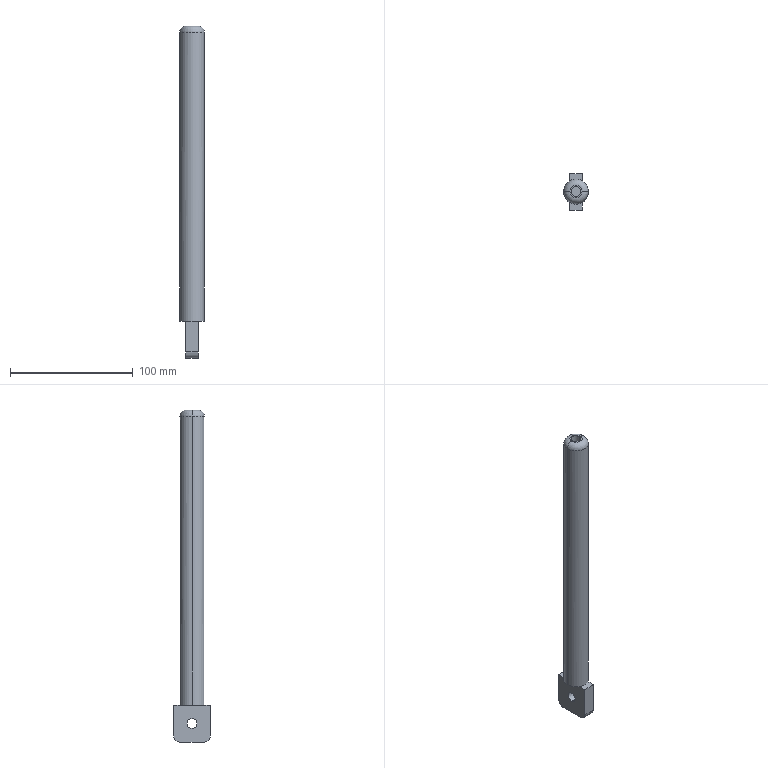Part | SolidWorks | features ICE 3, Fillet 2, Extrusion 1 | 1 solid | 21 faces | box 20 x 30 x 270 mm | volume 82484 mm3 | plane 11 | cylinder 8 | torus 2 | commonest cylinder face diameters 8 x4 10 x2 20 x2
STEP:
#1=CARTESIAN_POINT('',(-4.,0.,220.));
#2=VERTEX_POINT('',#1);
#3=CARTESIAN_POINT('',(4.,0.,220.));
#4=VERTEX_POINT('',#3);
#5=CARTESIAN_POINT('',(0.,0.,220.));
#6=DIRECTION('',(0.,0.,1.));
#7=DIRECTION('',(1.,0.,0.));
#8=AXIS2_PLACEMENT_3D('',#5,#6,#7);
#9=CIRCLE('',#8,4.);
#10=EDGE_CURVE('',#2,#4,#9,.T.);
#11=ORIENTED_EDGE('',*,*,#10,.F.);
#12=CARTESIAN_POINT('',(-4.,0.,240.));
#13=VERTEX_POINT('',#12);
#14=CARTESIAN_POINT('',(-4.,0.,220.));
#15=DIRECTION('',(0.,0.,1.));
#16=VECTOR('',#15,1000.);
#17=LINE('',#14,#16);
#18=EDGE_CURVE('',#2,#13,#17,.T.);
#19=ORIENTED_EDGE('',*,*,#18,.T.);
#20=CARTESIAN_POINT('',(4.,0.,240.));
#21=VERTEX_POINT('',#20);
#22=CARTESIAN_POINT('',(0.,0.,240.));
#23=DIRECTION('',(0.,0.,1.));
#24=DIRECTION('',(1.,0.,0.));
#25=AXIS2_PLACEMENT_3D('',#22,#23,#24);
#26=CIRCLE('',#25,4.);
#27=EDGE_CURVE('',#13,#21,#26,.T.);
#28=ORIENTED_EDGE('',*,*,#27,.T.);
#29=CARTESIAN_POINT('',(4.,0.,220.));
#30=DIRECTION('',(0.,0.,1.));
#31=VECTOR('',#30,1000.);
#32=LINE('',#29,#31);
#33=EDGE_CURVE('',#4,#21,#32,.T.);
#34=ORIENTED_EDGE('',*,*,#33,.F.);
#35=EDGE_LOOP('',(#11,#19,#28,#34));
#36=FACE_OUTER_BOUND('',#35,.T.);
#37=CARTESIAN_POINT('',(0.,0.,220.));
#38=DIRECTION('',(0.,0.,1.));
#39=DIRECTION('',(1.,0.,0.));
#40=AXIS2_PLACEMENT_3D('',#37,#38,#39);
#41=CYLINDRICAL_SURFACE('',#40,4.);
#42=ADVANCED_FACE('',(#36),#41,.F.);
#43=CARTESIAN_POINT('',(-10.,0.,235.));
#44=VERTEX_POINT('',#43);
#45=CARTESIAN_POINT('',(10.,0.,235.));
#46=VERTEX_POINT('',#45);
#47=CARTESIAN_POINT('',(0.,0.,235.));
#48=DIRECTION('',(0.,0.,-1.));
#49=DIRECTION('',(1.,0.,0.));
#50=AXIS2_PLACEMENT_3D('',#47,#48,#49);
#51=CIRCLE('',#50,10.);
#52=EDGE_CURVE('',#44,#46,#51,.T.);
#53=ORIENTED_EDGE('',*,*,#52,.F.);
#54=CARTESIAN_POINT('',(-5.,0.,240.));
#55=VERTEX_POINT('',#54);
#56=CARTESIAN_POINT('',(-5.,0.,235.));
#57=DIRECTION('',(0.,1.,0.));
#58=DIRECTION('',(-1.,0.,0.));
#59=AXIS2_PLACEMENT_3D('',#56,#57,#58);
#60=CIRCLE('',#59,5.);
#61=EDGE_CURVE('',#44,#55,#60,.T.);
#62=ORIENTED_EDGE('',*,*,#61,.T.);
#63=CARTESIAN_POINT('',(5.,0.,240.));
#64=VERTEX_POINT('',#63);
#65=CARTESIAN_POINT('',(0.,0.,240.));
#66=DIRECTION('',(0.,0.,1.));
#67=DIRECTION('',(1.,0.,0.));
#68=AXIS2_PLACEMENT_3D('',#65,#66,#67);
#69=CIRCLE('',#68,5.);
#70=EDGE_CURVE('',#64,#55,#69,.T.);
#71=ORIENTED_EDGE('',*,*,#70,.F.);
#72=CARTESIAN_POINT('',(5.,0.,235.));
#73=DIRECTION('',(0.,-1.,0.));
#74=DIRECTION('',(0.,0.,-1.));
#75=AXIS2_PLACEMENT_3D('',#72,#73,#74);
#76=CIRCLE('',#75,5.);
#77=EDGE_CURVE('',#46,#64,#76,.T.);
#78=ORIENTED_EDGE('',*,*,#77,.F.);
#79=EDGE_LOOP('',(#53,#62,#71,#78));
#80=FACE_OUTER_BOUND('',#79,.T.);
#81=CARTESIAN_POINT('',(0.,0.,235.));
#82=DIRECTION('',(0.,0.,1.));
#83=DIRECTION('',(1.,0.,0.));
#84=AXIS2_PLACEMENT_3D('',#81,#82,#83);
#85=TOROIDAL_SURFACE('',#84,5.,5.);
#86=ADVANCED_FACE('',(#80),#85,.T.);
#87=CARTESIAN_POINT('',(-5.,0.,-19.));
#88=VERTEX_POINT('',#87);
#89=CARTESIAN_POINT('',(-5.,0.,-11.));
#90=VERTEX_POINT('',#89);
#91=CARTESIAN_POINT('',(-5.,0.,-15.));
#92=DIRECTION('',(-1.,0.,0.));
#93=DIRECTION('',(0.,0.,1.));
#94=AXIS2_PLACEMENT_3D('',#91,#92,#93);
#95=CIRCLE('',#94,4.);
#96=EDGE_CURVE('',#88,#90,#95,.T.);
#97=ORIENTED_EDGE('',*,*,#96,.T.);
#98=CARTESIAN_POINT('',(5.,0.,-11.));
#99=VERTEX_POINT('',#98);
#100=CARTESIAN_POINT('',(-33.,0.,-11.));
#101=DIRECTION('',(1.,0.,0.));
#102=VECTOR('',#101,1000.);
#103=LINE('',#100,#102);
#104=EDGE_CURVE('',#90,#99,#103,.T.);
#105=ORIENTED_EDGE('',*,*,#104,.T.);
#106=CARTESIAN_POINT('',(5.,0.,-19.));
#107=VERTEX_POINT('',#106);
#108=CARTESIAN_POINT('',(5.,0.,-15.));
#109=DIRECTION('',(1.,0.,0.));
#110=DIRECTION('',(0.,0.,-1.));
#111=AXIS2_PLACEMENT_3D('',#108,#109,#110);
#112=CIRCLE('',#111,4.);
#113=EDGE_CURVE('',#99,#107,#112,.T.);
#114=ORIENTED_EDGE('',*,*,#113,.T.);
#115=CARTESIAN_POINT('',(-33.,0.,-19.));
#116=DIRECTION('',(1.,0.,0.));
#117=VECTOR('',#116,1000.);
#118=LINE('',#115,#117);
#119=EDGE_CURVE('',#88,#107,#118,.T.);
#120=ORIENTED_EDGE('',*,*,#119,.F.);
#121=EDGE_LOOP('',(#97,#105,#114,#120));
#122=FACE_OUTER_BOUND('',#121,.T.);
#123=CARTESIAN_POINT('',(-33.,0.,-15.));
#124=DIRECTION('',(1.,0.,0.));
#125=DIRECTION('',(0.,0.,-1.));
#126=AXIS2_PLACEMENT_3D('',#123,#124,#125);
#127=CYLINDRICAL_SURFACE('',#126,4.);
#128=ADVANCED_FACE('',(#122),#127,.F.);
#129=ORIENTED_EDGE('',*,*,#52,.T.);
#130=CARTESIAN_POINT('',(10.,0.,0.));
#131=VERTEX_POINT('',#130);
#132=CARTESIAN_POINT('',(10.,0.,240.));
#133=DIRECTION('',(0.,0.,-1.));
#134=VECTOR('',#133,1000.);
#135=LINE('',#132,#134);
#136=EDGE_CURVE('',#46,#131,#135,.T.);
#137=ORIENTED_EDGE('',*,*,#136,.T.);
#138=CARTESIAN_POINT('',(5.,8.66,0.));
#139=VERTEX_POINT('',#138);
#140=CARTESIAN_POINT('',(0.,0.,0.));
#141=DIRECTION('',(0.,0.,1.));
#142=DIRECTION('',(1.,0.,0.));
#143=AXIS2_PLACEMENT_3D('',#140,#141,#142);
#144=CIRCLE('',#143,10.);
#145=EDGE_CURVE('',#131,#139,#144,.T.);
#146=ORIENTED_EDGE('',*,*,#145,.T.);
#147=CARTESIAN_POINT('',(-5.,8.66,0.));
#148=VERTEX_POINT('',#147);
#149=CARTESIAN_POINT('',(0.,0.,0.));
#150=DIRECTION('',(0.,0.,1.));
#151=DIRECTION('',(1.,0.,0.));
#152=AXIS2_PLACEMENT_3D('',#149,#150,#151);
#153=CIRCLE('',#152,10.);
#154=EDGE_CURVE('',#139,#148,#153,.T.);
#155=ORIENTED_EDGE('',*,*,#154,.T.);
#156=CARTESIAN_POINT('',(-10.,0.,0.));
#157=VERTEX_POINT('',#156);
#158=CARTESIAN_POINT('',(0.,0.,0.));
#159=DIRECTION('',(0.,0.,1.));
#160=DIRECTION('',(1.,0.,0.));
#161=AXIS2_PLACEMENT_3D('',#158,#159,#160);
#162=CIRCLE('',#161,10.);
#163=EDGE_CURVE('',#148,#157,#162,.T.);
#164=ORIENTED_EDGE('',*,*,#163,.T.);
#165=CARTESIAN_POINT('',(-10.,0.,240.));
#166=DIRECTION('',(0.,0.,-1.));
#167=VECTOR('',#166,1000.);
#168=LINE('',#165,#167);
#169=EDGE_CURVE('',#44,#157,#168,.T.);
#170=ORIENTED_EDGE('',*,*,#169,.F.);
#171=EDGE_LOOP('',(#129,#137,#146,#155,#164,#170));
#172=FACE_OUTER_BOUND('',#171,.T.);
#173=CARTESIAN_POINT('',(0.,0.,240.));
#174=DIRECTION('',(0.,0.,-1.));
#175=DIRECTION('',(-1.,0.,0.));
#176=AXIS2_PLACEMENT_3D('',#173,#174,#175);
#177=CYLINDRICAL_SURFACE('',#176,10.);
#178=ADVANCED_FACE('',(#172),#177,.T.);
#179=CARTESIAN_POINT('',(5.,-8.66,0.));
#180=VERTEX_POINT('',#179);
#181=CARTESIAN_POINT('',(5.,-15.,0.));
#182=DIRECTION('',(0.,-1.,0.));
#183=VECTOR('',#182,1000.);
#184=LINE('',#181,#183);
#185=EDGE_CURVE('',#139,#180,#184,.T.);
#186=ORIENTED_EDGE('',*,*,#185,.F.);
#187=ORIENTED_EDGE('',*,*,#145,.F.);
#188=CARTESIAN_POINT('',(0.,0.,0.));
#189=DIRECTION('',(0.,0.,1.));
#190=DIRECTION('',(1.,0.,0.));
#191=AXIS2_PLACEMENT_3D('',#188,#189,#190);
#192=CIRCLE('',#191,10.);
#193=EDGE_CURVE('',#180,#131,#192,.T.);
#194=ORIENTED_EDGE('',*,*,#193,.F.);
#195=EDGE_LOOP('',(#186,#187,#194));
#196=FACE_OUTER_BOUND('',#195,.T.);
#197=CARTESIAN_POINT('',(0.,0.,0.));
#198=DIRECTION('',(0.,0.,1.));
#199=DIRECTION('',(1.,0.,0.));
#200=AXIS2_PLACEMENT_3D('',#197,#198,#199);
#201=PLANE('',#200);
#202=ADVANCED_FACE('',(#196),#201,.F.);
#203=ORIENTED_EDGE('',*,*,#136,.F.);
#204=CARTESIAN_POINT('',(0.,0.,235.));
#205=DIRECTION('',(0.,0.,-1.));
#206=DIRECTION('',(1.,0.,0.));
#207=AXIS2_PLACEMENT_3D('',#204,#205,#206);
#208=CIRCLE('',#207,10.);
#209=EDGE_CURVE('',#46,#44,#208,.T.);
#210=ORIENTED_EDGE('',*,*,#209,.T.);
#211=ORIENTED_EDGE('',*,*,#169,.T.);
#212=CARTESIAN_POINT('',(-5.,-8.66,0.));
#213=VERTEX_POINT('',#212);
#214=CARTESIAN_POINT('',(0.,0.,0.));
#215=DIRECTION('',(0.,0.,1.));
#216=DIRECTION('',(1.,0.,0.));
#217=AXIS2_PLACEMENT_3D('',#214,#215,#216);
#218=CIRCLE('',#217,10.);
#219=EDGE_CURVE('',#157,#213,#218,.T.);
#220=ORIENTED_EDGE('',*,*,#219,.T.);
#221=CARTESIAN_POINT('',(0.,0.,0.));
#222=DIRECTION('',(0.,0.,1.));
#223=DIRECTION('',(1.,0.,0.));
#224=AXIS2_PLACEMENT_3D('',#221,#222,#223);
#225=CIRCLE('',#224,10.);
#226=EDGE_CURVE('',#213,#180,#225,.T.);
#227=ORIENTED_EDGE('',*,*,#226,.T.);
#228=ORIENTED_EDGE('',*,*,#193,.T.);
#229=EDGE_LOOP('',(#203,#210,#211,#220,#227,#228));
#230=FACE_OUTER_BOUND('',#229,.T.);
#231=CARTESIAN_POINT('',(0.,0.,240.));
#232=DIRECTION('',(0.,0.,-1.));
#233=DIRECTION('',(-1.,0.,0.));
#234=AXIS2_PLACEMENT_3D('',#231,#232,#233);
#235=CYLINDRICAL_SURFACE('',#234,10.);
#236=ADVANCED_FACE('',(#230),#235,.T.);
#237=CARTESIAN_POINT('',(0.,0.,240.));
#238=DIRECTION('',(0.,0.,1.));
#239=DIRECTION('',(1.,0.,0.));
#240=AXIS2_PLACEMENT_3D('',#237,#238,#239);
#241=CIRCLE('',#240,4.);
#242=EDGE_CURVE('',#21,#13,#241,.T.);
#243=ORIENTED_EDGE('',*,*,#242,.F.);
#244=ORIENTED_EDGE('',*,*,#27,.F.);
#245=EDGE_LOOP('',(#243,#244));
#246=FACE_BOUND('',#245,.T.);
#247=ORIENTED_EDGE('',*,*,#70,.T.);
#248=CARTESIAN_POINT('',(0.,0.,240.));
#249=DIRECTION('',(0.,0.,1.));
#250=DIRECTION('',(1.,0.,0.));
#251=AXIS2_PLACEMENT_3D('',#248,#249,#250);
#252=CIRCLE('',#251,5.);
#253=EDGE_CURVE('',#55,#64,#252,.T.);
#254=ORIENTED_EDGE('',*,*,#253,.T.);
#255=EDGE_LOOP('',(#247,#254));
#256=FACE_OUTER_BOUND('',#255,.T.);
#257=CARTESIAN_POINT('',(0.,0.,240.));
#258=DIRECTION('',(0.,0.,1.));
#259=DIRECTION('',(1.,0.,0.));
#260=AXIS2_PLACEMENT_3D('',#257,#258,#259);
#261=PLANE('',#260);
#262=ADVANCED_FACE('',(#246,#256),#261,.T.);
#263=ORIENTED_EDGE('',*,*,#163,.F.);
#264=CARTESIAN_POINT('',(-5.,-15.,0.));
#265=DIRECTION('',(0.,-1.,0.));
#266=VECTOR('',#265,1000.);
#267=LINE('',#264,#266);
#268=EDGE_CURVE('',#148,#213,#267,.T.);
#269=ORIENTED_EDGE('',*,*,#268,.T.);
#270=ORIENTED_EDGE('',*,*,#219,.F.);
#271=EDGE_LOOP('',(#263,#269,#270));
#272=FACE_OUTER_BOUND('',#271,.T.);
#273=CARTESIAN_POINT('',(0.,0.,0.));
#274=DIRECTION('',(0.,0.,1.));
#275=DIRECTION('',(1.,0.,0.));
#276=AXIS2_PLACEMENT_3D('',#273,#274,#275);
#277=PLANE('',#276);
#278=ADVANCED_FACE('',(#272),#277,.F.);
#279=ORIENTED_EDGE('',*,*,#154,.F.);
#280=CARTESIAN_POINT('',(5.,15.,0.));
#281=VERTEX_POINT('',#280);
#282=CARTESIAN_POINT('',(5.,-15.,0.));
#283=DIRECTION('',(0.,-1.,0.));
#284=VECTOR('',#283,1000.);
#285=LINE('',#282,#284);
#286=EDGE_CURVE('',#281,#139,#285,.T.);
#287=ORIENTED_EDGE('',*,*,#286,.F.);
#288=CARTESIAN_POINT('',(-5.,15.,0.));
#289=VERTEX_POINT('',#288);
#290=CARTESIAN_POINT('',(5.,15.,0.));
#291=DIRECTION('',(-1.,0.,0.));
#292=VECTOR('',#291,1000.);
#293=LINE('',#290,#292);
#294=EDGE_CURVE('',#281,#289,#293,.T.);
#295=ORIENTED_EDGE('',*,*,#294,.T.);
#296=CARTESIAN_POINT('',(-5.,-15.,0.));
#297=DIRECTION('',(0.,-1.,0.));
#298=VECTOR('',#297,1000.);
#299=LINE('',#296,#298);
#300=EDGE_CURVE('',#289,#148,#299,.T.);
#301=ORIENTED_EDGE('',*,*,#300,.T.);
#302=EDGE_LOOP('',(#279,#287,#295,#301));
#303=FACE_OUTER_BOUND('',#302,.T.);
#304=CARTESIAN_POINT('',(5.,-15.,0.));
#305=DIRECTION('',(0.,0.,-1.));
#306=DIRECTION('',(-1.,0.,0.));
#307=AXIS2_PLACEMENT_3D('',#304,#305,#306);
#308=PLANE('',#307);
#309=ADVANCED_FACE('',(#303),#308,.F.);
#310=CARTESIAN_POINT('',(-5.,-10.,-30.));
#311=VERTEX_POINT('',#310);
#312=CARTESIAN_POINT('',(-5.,10.,-30.));
#313=VERTEX_POINT('',#312);
#314=CARTESIAN_POINT('',(-5.,-15.,-30.));
#315=DIRECTION('',(0.,1.,0.));
#316=VECTOR('',#315,1000.);
#317=LINE('',#314,#316);
#318=EDGE_CURVE('',#311,#313,#317,.T.);
#319=ORIENTED_EDGE('',*,*,#318,.T.);
#320=CARTESIAN_POINT('',(5.,10.,-30.));
#321=VERTEX_POINT('',#320);
#322=CARTESIAN_POINT('',(5.,10.,-30.));
#323=DIRECTION('',(1.,0.,0.));
#324=VECTOR('',#323,1000.);
#325=LINE('',#322,#324);
#326=EDGE_CURVE('',#313,#321,#325,.T.);
#327=ORIENTED_EDGE('',*,*,#326,.T.);
#328=CARTESIAN_POINT('',(5.,-10.,-30.));
#329=VERTEX_POINT('',#328);
#330=CARTESIAN_POINT('',(5.,-15.,-30.));
#331=DIRECTION('',(0.,1.,0.));
#332=VECTOR('',#331,1000.);
#333=LINE('',#330,#332);
#334=EDGE_CURVE('',#329,#321,#333,.T.);
#335=ORIENTED_EDGE('',*,*,#334,.F.);
#336=CARTESIAN_POINT('',(5.,-10.,-30.));
#337=DIRECTION('',(-1.,0.,0.));
#338=VECTOR('',#337,1000.);
#339=LINE('',#336,#338);
#340=EDGE_CURVE('',#329,#311,#339,.T.);
#341=ORIENTED_EDGE('',*,*,#340,.T.);
#342=EDGE_LOOP('',(#319,#327,#335,#341));
#343=FACE_OUTER_BOUND('',#342,.T.);
#344=CARTESIAN_POINT('',(5.,-15.,-30.));
#345=DIRECTION('',(0.,0.,1.));
#346=DIRECTION('',(1.,0.,0.));
#347=AXIS2_PLACEMENT_3D('',#344,#345,#346);
#348=PLANE('',#347);
#349=ADVANCED_FACE('',(#343),#348,.F.);
#350=CARTESIAN_POINT('',(5.,15.,-25.));
#351=VERTEX_POINT('',#350);
#352=CARTESIAN_POINT('',(5.,15.,0.));
#353=DIRECTION('',(0.,0.,1.));
#354=VECTOR('',#353,1000.);
#355=LINE('',#352,#354);
#356=EDGE_CURVE('',#351,#281,#355,.T.);
#357=ORIENTED_EDGE('',*,*,#356,.F.);
#358=CARTESIAN_POINT('',(-5.,15.,-25.));
#359=VERTEX_POINT('',#358);
#360=CARTESIAN_POINT('',(5.,15.,-25.));
#361=DIRECTION('',(-1.,0.,0.));
#362=VECTOR('',#361,1000.);
#363=LINE('',#360,#362);
#364=EDGE_CURVE('',#351,#359,#363,.T.);
#365=ORIENTED_EDGE('',*,*,#364,.T.);
#366=CARTESIAN_POINT('',(-5.,15.,0.));
#367=DIRECTION('',(0.,0.,1.));
#368=VECTOR('',#367,1000.);
#369=LINE('',#366,#368);
#370=EDGE_CURVE('',#359,#289,#369,.T.);
#371=ORIENTED_EDGE('',*,*,#370,.T.);
#372=ORIENTED_EDGE('',*,*,#294,.F.);
#373=EDGE_LOOP('',(#357,#365,#371,#372));
#374=FACE_OUTER_BOUND('',#373,.T.);
#375=CARTESIAN_POINT('',(5.,15.,0.));
#376=DIRECTION('',(0.,-1.,0.));
#377=DIRECTION('',(0.,0.,-1.));
#378=AXIS2_PLACEMENT_3D('',#375,#376,#377);
#379=PLANE('',#378);
#380=ADVANCED_FACE('',(#374),#379,.F.);
#381=ORIENTED_EDGE('',*,*,#226,.F.);
#382=CARTESIAN_POINT('',(-5.,-15.,0.));
#383=VERTEX_POINT('',#382);
#384=CARTESIAN_POINT('',(-5.,-15.,0.));
#385=DIRECTION('',(0.,-1.,0.));
#386=VECTOR('',#385,1000.);
#387=LINE('',#384,#386);
#388=EDGE_CURVE('',#213,#383,#387,.T.);
#389=ORIENTED_EDGE('',*,*,#388,.T.);
#390=CARTESIAN_POINT('',(5.,-15.,0.));
#391=VERTEX_POINT('',#390);
#392=CARTESIAN_POINT('',(5.,-15.,0.));
#393=DIRECTION('',(-1.,0.,0.));
#394=VECTOR('',#393,1000.);
#395=LINE('',#392,#394);
#396=EDGE_CURVE('',#391,#383,#395,.T.);
#397=ORIENTED_EDGE('',*,*,#396,.F.);
#398=CARTESIAN_POINT('',(5.,-15.,0.));
#399=DIRECTION('',(0.,-1.,0.));
#400=VECTOR('',#399,1000.);
#401=LINE('',#398,#400);
#402=EDGE_CURVE('',#180,#391,#401,.T.);
#403=ORIENTED_EDGE('',*,*,#402,.F.);
#404=EDGE_LOOP('',(#381,#389,#397,#403));
#405=FACE_OUTER_BOUND('',#404,.T.);
#406=CARTESIAN_POINT('',(5.,-15.,0.));
#407=DIRECTION('',(0.,0.,-1.));
#408=DIRECTION('',(-1.,0.,0.));
#409=AXIS2_PLACEMENT_3D('',#406,#407,#408);
#410=PLANE('',#409);
#411=ADVANCED_FACE('',(#405),#410,.F.);
#412=CARTESIAN_POINT('',(-5.,-15.,-25.));
#413=VERTEX_POINT('',#412);
#414=CARTESIAN_POINT('',(-5.,-15.,0.));
#415=DIRECTION('',(0.,0.,-1.));
#416=VECTOR('',#415,1000.);
#417=LINE('',#414,#416);
#418=EDGE_CURVE('',#383,#413,#417,.T.);
#419=ORIENTED_EDGE('',*,*,#418,.T.);
#420=CARTESIAN_POINT('',(5.,-15.,-25.));
#421=VERTEX_POINT('',#420);
#422=CARTESIAN_POINT('',(5.,-15.,-25.));
#423=DIRECTION('',(1.,0.,0.));
#424=VECTOR('',#423,1000.);
#425=LINE('',#422,#424);
#426=EDGE_CURVE('',#413,#421,#425,.T.);
#427=ORIENTED_EDGE('',*,*,#426,.T.);
#428=CARTESIAN_POINT('',(5.,-15.,0.));
#429=DIRECTION('',(0.,0.,-1.));
#430=VECTOR('',#429,1000.);
#431=LINE('',#428,#430);
#432=EDGE_CURVE('',#391,#421,#431,.T.);
#433=ORIENTED_EDGE('',*,*,#432,.F.);
#434=ORIENTED_EDGE('',*,*,#396,.T.);
#435=EDGE_LOOP('',(#419,#427,#433,#434));
#436=FACE_OUTER_BOUND('',#435,.T.);
#437=CARTESIAN_POINT('',(5.,-15.,0.));
#438=DIRECTION('',(0.,1.,0.));
#439=DIRECTION('',(0.,0.,1.));
#440=AXIS2_PLACEMENT_3D('',#437,#438,#439);
#441=PLANE('',#440);
#442=ADVANCED_FACE('',(#436),#441,.F.);
#443=CARTESIAN_POINT('',(5.,0.,-15.));
#444=DIRECTION('',(1.,0.,0.));
#445=DIRECTION('',(0.,0.,-1.));
#446=AXIS2_PLACEMENT_3D('',#443,#444,#445);
#447=CIRCLE('',#446,4.);
#448=EDGE_CURVE('',#107,#99,#447,.T.);
#449=ORIENTED_EDGE('',*,*,#448,.F.);
#450=ORIENTED_EDGE('',*,*,#113,.F.);
#451=EDGE_LOOP('',(#449,#450));
#452=FACE_BOUND('',#451,.T.);
#453=ORIENTED_EDGE('',*,*,#334,.T.);
#454=CARTESIAN_POINT('',(5.,10.,-25.));
#455=DIRECTION('',(1.,0.,0.));
#456=DIRECTION('',(0.,0.,1.));
#457=AXIS2_PLACEMENT_3D('',#454,#455,#456);
#458=CIRCLE('',#457,5.);
#459=EDGE_CURVE('',#321,#351,#458,.T.);
#460=ORIENTED_EDGE('',*,*,#459,.T.);
#461=ORIENTED_EDGE('',*,*,#356,.T.);
#462=ORIENTED_EDGE('',*,*,#286,.T.);
#463=ORIENTED_EDGE('',*,*,#185,.T.);
#464=ORIENTED_EDGE('',*,*,#402,.T.);
#465=ORIENTED_EDGE('',*,*,#432,.T.);
#466=CARTESIAN_POINT('',(5.,-10.,-25.));
#467=DIRECTION('',(1.,0.,0.));
#468=DIRECTION('',(0.,0.,1.));
#469=AXIS2_PLACEMENT_3D('',#466,#467,#468);
#470=CIRCLE('',#469,5.);
#471=EDGE_CURVE('',#421,#329,#470,.T.);
#472=ORIENTED_EDGE('',*,*,#471,.T.);
#473=EDGE_LOOP('',(#453,#460,#461,#462,#463,#464,#465,#472));
#474=FACE_OUTER_BOUND('',#473,.T.);
#475=CARTESIAN_POINT('',(5.,0.,0.));
#476=DIRECTION('',(-1.,0.,0.));
#477=DIRECTION('',(0.,0.,1.));
#478=AXIS2_PLACEMENT_3D('',#475,#476,#477);
#479=PLANE('',#478);
#480=ADVANCED_FACE('',(#452,#474),#479,.F.);
#481=ORIENTED_EDGE('',*,*,#96,.F.);
#482=CARTESIAN_POINT('',(-5.,0.,-15.));
#483=DIRECTION('',(-1.,0.,0.));
#484=DIRECTION('',(0.,0.,1.));
#485=AXIS2_PLACEMENT_3D('',#482,#483,#484);
#486=CIRCLE('',#485,4.);
#487=EDGE_CURVE('',#90,#88,#486,.T.);
#488=ORIENTED_EDGE('',*,*,#487,.F.);
#489=EDGE_LOOP('',(#481,#488));
#490=FACE_BOUND('',#489,.T.);
#491=ORIENTED_EDGE('',*,*,#370,.F.);
#492=CARTESIAN_POINT('',(-5.,10.,-25.));
#493=DIRECTION('',(-1.,0.,0.));
#494=DIRECTION('',(0.,0.,1.));
#495=AXIS2_PLACEMENT_3D('',#492,#493,#494);
#496=CIRCLE('',#495,5.);
#497=EDGE_CURVE('',#359,#313,#496,.T.);
#498=ORIENTED_EDGE('',*,*,#497,.T.);
#499=ORIENTED_EDGE('',*,*,#318,.F.);
#500=CARTESIAN_POINT('',(-5.,-10.,-25.));
#501=DIRECTION('',(-1.,0.,0.));
#502=DIRECTION('',(0.,0.,1.));
#503=AXIS2_PLACEMENT_3D('',#500,#501,#502);
#504=CIRCLE('',#503,5.);
#505=EDGE_CURVE('',#311,#413,#504,.T.);
#506=ORIENTED_EDGE('',*,*,#505,.T.);
#507=ORIENTED_EDGE('',*,*,#418,.F.);
#508=ORIENTED_EDGE('',*,*,#388,.F.);
#509=ORIENTED_EDGE('',*,*,#268,.F.);
#510=ORIENTED_EDGE('',*,*,#300,.F.);
#511=EDGE_LOOP('',(#491,#498,#499,#506,#507,#508,#509,#510));
#512=FACE_OUTER_BOUND('',#511,.T.);
#513=CARTESIAN_POINT('',(-5.,0.,0.));
#514=DIRECTION('',(-1.,0.,0.));
#515=DIRECTION('',(0.,0.,1.));
#516=AXIS2_PLACEMENT_3D('',#513,#514,#515);
#517=PLANE('',#516);
#518=ADVANCED_FACE('',(#490,#512),#517,.T.);
#519=ORIENTED_EDGE('',*,*,#104,.F.);
#520=ORIENTED_EDGE('',*,*,#487,.T.);
#521=ORIENTED_EDGE('',*,*,#119,.T.);
#522=ORIENTED_EDGE('',*,*,#448,.T.);
#523=EDGE_LOOP('',(#519,#520,#521,#522));
#524=FACE_OUTER_BOUND('',#523,.T.);
#525=CARTESIAN_POINT('',(-33.,0.,-15.));
#526=DIRECTION('',(1.,0.,0.));
#527=DIRECTION('',(0.,0.,-1.));
#528=AXIS2_PLACEMENT_3D('',#525,#526,#527);
#529=CYLINDRICAL_SURFACE('',#528,4.);
#530=ADVANCED_FACE('',(#524),#529,.F.);
#531=ORIENTED_EDGE('',*,*,#459,.F.);
#532=ORIENTED_EDGE('',*,*,#326,.F.);
#533=ORIENTED_EDGE('',*,*,#497,.F.);
#534=ORIENTED_EDGE('',*,*,#364,.F.);
#535=EDGE_LOOP('',(#531,#532,#533,#534));
#536=FACE_OUTER_BOUND('',#535,.T.);
#537=CARTESIAN_POINT('',(5.,10.,-25.));
#538=DIRECTION('',(-1.,0.,0.));
#539=DIRECTION('',(0.,0.,1.));
#540=AXIS2_PLACEMENT_3D('',#537,#538,#539);
#541=CYLINDRICAL_SURFACE('',#540,5.);
#542=ADVANCED_FACE('',(#536),#541,.T.);
#543=ORIENTED_EDGE('',*,*,#471,.F.);
#544=ORIENTED_EDGE('',*,*,#426,.F.);
#545=ORIENTED_EDGE('',*,*,#505,.F.);
#546=ORIENTED_EDGE('',*,*,#340,.F.);
#547=EDGE_LOOP('',(#543,#544,#545,#546));
#548=FACE_OUTER_BOUND('',#547,.T.);
#549=CARTESIAN_POINT('',(5.,-10.,-25.));
#550=DIRECTION('',(-1.,0.,0.));
#551=DIRECTION('',(0.,0.,1.));
#552=AXIS2_PLACEMENT_3D('',#549,#550,#551);
#553=CYLINDRICAL_SURFACE('',#552,5.);
#554=ADVANCED_FACE('',(#548),#553,.T.);
#555=ORIENTED_EDGE('',*,*,#61,.F.);
#556=ORIENTED_EDGE('',*,*,#209,.F.);
#557=ORIENTED_EDGE('',*,*,#77,.T.);
#558=ORIENTED_EDGE('',*,*,#253,.F.);
#559=EDGE_LOOP('',(#555,#556,#557,#558));
#560=FACE_OUTER_BOUND('',#559,.T.);
#561=CARTESIAN_POINT('',(0.,0.,235.));
#562=DIRECTION('',(0.,0.,1.));
#563=DIRECTION('',(1.,0.,0.));
#564=AXIS2_PLACEMENT_3D('',#561,#562,#563);
#565=TOROIDAL_SURFACE('',#564,5.,5.);
#566=ADVANCED_FACE('',(#560),#565,.T.);
#567=ORIENTED_EDGE('',*,*,#18,.F.);
#568=CARTESIAN_POINT('',(0.,0.,220.));
#569=DIRECTION('',(0.,0.,1.));
#570=DIRECTION('',(1.,0.,0.));
#571=AXIS2_PLACEMENT_3D('',#568,#569,#570);
#572=CIRCLE('',#571,4.);
#573=EDGE_CURVE('',#4,#2,#572,.T.);
#574=ORIENTED_EDGE('',*,*,#573,.F.);
#575=ORIENTED_EDGE('',*,*,#33,.T.);
#576=ORIENTED_EDGE('',*,*,#242,.T.);
#577=EDGE_LOOP('',(#567,#574,#575,#576));
#578=FACE_OUTER_BOUND('',#577,.T.);
#579=CARTESIAN_POINT('',(0.,0.,220.));
#580=DIRECTION('',(0.,0.,1.));
#581=DIRECTION('',(1.,0.,0.));
#582=AXIS2_PLACEMENT_3D('',#579,#580,#581);
#583=CYLINDRICAL_SURFACE('',#582,4.);
#584=ADVANCED_FACE('',(#578),#583,.F.);
#585=ORIENTED_EDGE('',*,*,#573,.T.);
#586=ORIENTED_EDGE('',*,*,#10,.T.);
#587=EDGE_LOOP('',(#585,#586));
#588=FACE_OUTER_BOUND('',#587,.T.);
#589=CARTESIAN_POINT('',(0.,0.,220.));
#590=DIRECTION('',(0.,0.,1.));
#591=DIRECTION('',(1.,0.,0.));
#592=AXIS2_PLACEMENT_3D('',#589,#590,#591);
#593=PLANE('',#592);
#594=ADVANCED_FACE('',(#588),#593,.T.);
#595=CLOSED_SHELL('',(#42,#86,#128,#178,#202,#236,#262,#278,#309,#349,#380,#411,#442,#480,#518,#530,#542,#554,#566,#584,#594));
#596=MANIFOLD_SOLID_BREP('',#595);
#597=CARTESIAN_POINT('',(0.,0.,0.));
#598=DIRECTION('',(0.,0.,1.));
#599=DIRECTION('',(1.,0.,0.));
#600=AXIS2_PLACEMENT_3D('',#597,#598,#599);
#601=(LENGTH_UNIT()NAMED_UNIT(*)SI_UNIT(.MILLI.,.METRE.));
#602=UNCERTAINTY_MEASURE_WITH_UNIT(LENGTH_MEASURE(0.00001),#601,'','');
#603=(NAMED_UNIT(*)PLANE_ANGLE_UNIT()SI_UNIT($,.RADIAN.));
#604=(NAMED_UNIT(*)SI_UNIT($,.STERADIAN.)SOLID_ANGLE_UNIT());
#605=(GEOMETRIC_REPRESENTATION_CONTEXT(3)GLOBAL_UNCERTAINTY_ASSIGNED_CONTEXT((#602))GLOBAL_UNIT_ASSIGNED_CONTEXT((#601,#603,#604))REPRESENTATION_CONTEXT('',''));
#606=ADVANCED_BREP_SHAPE_REPRESENTATION('',(#596,#600),#605);